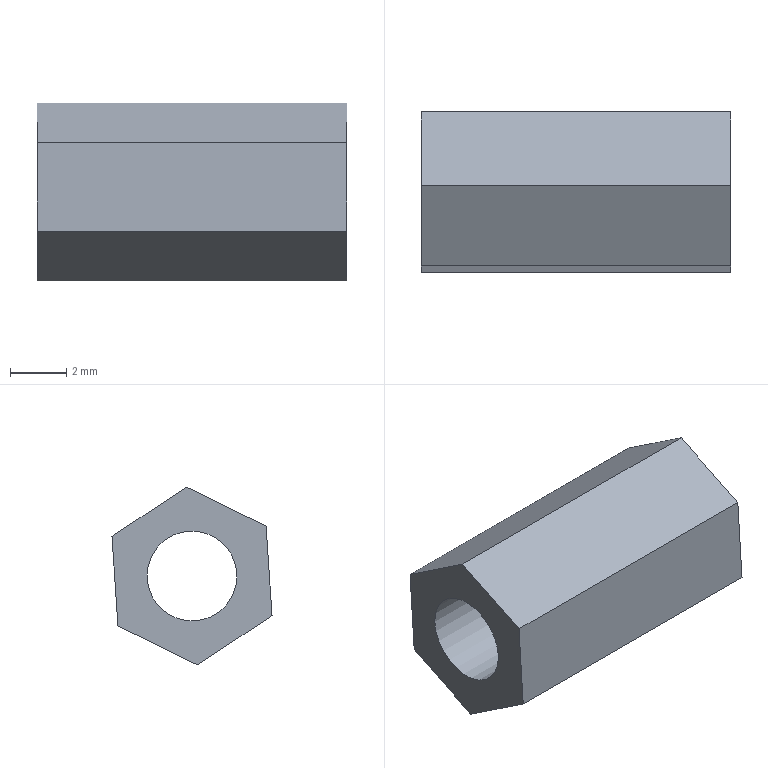Part | STEP file | Dodanie-wyci_gni_cie1_8 | 1 solid | 9 faces | box 11 x 5.689 x 6.325 mm | volume 198.638 mm3 | plane 8 | cylinder 1 | commonest cylinder face diameters 3.2 x1
STEP:
#1=CARTESIAN_POINT('',(0.,0.,0.));
#2=DIRECTION('',(0.,0.,1.));
#3=DIRECTION('',(1.,0.,0.));
#4=AXIS2_PLACEMENT_3D('',#1,#2,#3);
#5=CARTESIAN_POINT('',(142.868,119.819,-66.664));
#6=VERTEX_POINT('',#5);
#7=CARTESIAN_POINT('',(142.868,118.383,-67.37));
#8=DIRECTION('',(1.,0.,0.));
#9=DIRECTION('',(0.,0.8975,0.441));
#10=AXIS2_PLACEMENT_3D('',#7,#8,#9);
#11=CIRCLE('',#10,1.6);
#12=CARTESIAN_POINT('',(142.868,118.383,-67.37));
#13=DIRECTION('',(1.,0.,0.));
#14=DIRECTION('',(0.,0.8975,0.441));
#15=AXIS2_PLACEMENT_3D('',#12,#13,#14);
#16=CYLINDRICAL_SURFACE('',#15,1.6);
#17=CARTESIAN_POINT('',(0.,0.));
#18=DIRECTION('',(1.,0.));
#19=VECTOR('',#18,1.);
#20=LINE('',#17,#19);
#21=(GEOMETRIC_REPRESENTATION_CONTEXT(2)PARAMETRIC_REPRESENTATION_CONTEXT()REPRESENTATION_CONTEXT('',''));
#22=DEFINITIONAL_REPRESENTATION('',(#20),#21);
#23=PCURVE('',#16,#22);
#24=CARTESIAN_POINT('',(142.868,118.383,-67.37));
#25=DIRECTION('',(-1.,0.,0.));
#26=DIRECTION('',(0.,-0.8975,-0.441));
#27=AXIS2_PLACEMENT_3D('',#24,#25,#26);
#28=PLANE('',#27);
#29=CARTESIAN_POINT('',(-1.6,0.));
#30=CARTESIAN_POINT('',(-1.6,2.771));
#31=CARTESIAN_POINT('',(0.8,1.386));
#32=CARTESIAN_POINT('',(3.2,0.));
#33=CARTESIAN_POINT('',(0.8,-1.386));
#34=CARTESIAN_POINT('',(-1.6,-2.771));
#35=CARTESIAN_POINT('',(-1.6,0.));
#36=(BOUNDED_CURVE()B_SPLINE_CURVE(2,(#29,#30,#31,#32,#33,#34,#35),.UNSPECIFIED.,.T.,.F.)B_SPLINE_CURVE_WITH_KNOTS((1,2,2,2,2,1),(-2.094,0.,2.094,4.189,6.283,8.378),.UNSPECIFIED.)CURVE()GEOMETRIC_REPRESENTATION_ITEM()RATIONAL_B_SPLINE_CURVE((1.,0.5,1.,0.5,1.,0.5,1.))REPRESENTATION_ITEM(''));
#37=(GEOMETRIC_REPRESENTATION_CONTEXT(2)PARAMETRIC_REPRESENTATION_CONTEXT()REPRESENTATION_CONTEXT('',''));
#38=DEFINITIONAL_REPRESENTATION('',(#36),#37);
#39=PCURVE('',#28,#38);
#40=SURFACE_CURVE('',#11,(#23,#39),.PCURVE_S1.);
#41=EDGE_CURVE('',#6,#6,#40,.T.);
#42=ORIENTED_EDGE('',*,*,#41,.T.);
#43=CARTESIAN_POINT('',(153.868,119.819,-66.664));
#44=VERTEX_POINT('',#43);
#45=CARTESIAN_POINT('',(153.868,119.819,-66.664));
#46=DIRECTION('',(-1.,0.,0.));
#47=VECTOR('',#46,1.);
#48=LINE('',#45,#47);
#49=CARTESIAN_POINT('',(6.283,11.));
#50=DIRECTION('',(0.,-1.));
#51=VECTOR('',#50,1.);
#52=LINE('',#49,#51);
#53=(GEOMETRIC_REPRESENTATION_CONTEXT(2)PARAMETRIC_REPRESENTATION_CONTEXT()REPRESENTATION_CONTEXT('',''));
#54=DEFINITIONAL_REPRESENTATION('',(#52),#53);
#55=PCURVE('',#16,#54);
#56=CARTESIAN_POINT('',(0.,11.));
#57=DIRECTION('',(0.,-1.));
#58=VECTOR('',#57,1.);
#59=LINE('',#56,#58);
#60=(GEOMETRIC_REPRESENTATION_CONTEXT(2)PARAMETRIC_REPRESENTATION_CONTEXT()REPRESENTATION_CONTEXT('',''));
#61=DEFINITIONAL_REPRESENTATION('',(#59),#60);
#62=PCURVE('',#16,#61);
#63=SEAM_CURVE('',#48,(#55,#62),.PCURVE_S1.);
#64=EDGE_CURVE('',#44,#6,#63,.T.);
#65=ORIENTED_EDGE('',*,*,#64,.F.);
#66=CARTESIAN_POINT('',(153.868,118.383,-67.37));
#67=DIRECTION('',(-1.,0.,0.));
#68=DIRECTION('',(0.,0.8975,0.441));
#69=AXIS2_PLACEMENT_3D('',#66,#67,#68);
#70=CIRCLE('',#69,1.6);
#71=CARTESIAN_POINT('',(6.283,11.));
#72=DIRECTION('',(-1.,0.));
#73=VECTOR('',#72,1.);
#74=LINE('',#71,#73);
#75=(GEOMETRIC_REPRESENTATION_CONTEXT(2)PARAMETRIC_REPRESENTATION_CONTEXT()REPRESENTATION_CONTEXT('',''));
#76=DEFINITIONAL_REPRESENTATION('',(#74),#75);
#77=PCURVE('',#16,#76);
#78=CARTESIAN_POINT('',(153.868,118.383,-67.37));
#79=DIRECTION('',(-1.,0.,0.));
#80=DIRECTION('',(0.,-0.8975,-0.441));
#81=AXIS2_PLACEMENT_3D('',#78,#79,#80);
#82=PLANE('',#81);
#83=CARTESIAN_POINT('',(0.,0.));
#84=DIRECTION('',(-1.,0.));
#85=AXIS2_PLACEMENT_2D('',#83,#84);
#86=CIRCLE('',#85,1.6);
#87=(GEOMETRIC_REPRESENTATION_CONTEXT(2)PARAMETRIC_REPRESENTATION_CONTEXT()REPRESENTATION_CONTEXT('',''));
#88=DEFINITIONAL_REPRESENTATION('',(#86),#87);
#89=PCURVE('',#82,#88);
#90=SURFACE_CURVE('',#70,(#77,#89),.PCURVE_S1.);
#91=EDGE_CURVE('',#44,#44,#90,.T.);
#92=ORIENTED_EDGE('',*,*,#91,.T.);
#93=ORIENTED_EDGE('',*,*,#64,.T.);
#94=EDGE_LOOP('',(#42,#65,#92,#93));
#95=FACE_BOUND('',#94,.F.);
#96=ADVANCED_FACE('',(#95),#16,.F.);
#97=ORIENTED_EDGE('',*,*,#91,.T.);
#98=EDGE_LOOP('',(#97));
#99=FACE_BOUND('',#98,.T.);
#100=CARTESIAN_POINT('',(153.868,115.75,-65.605));
#101=VERTEX_POINT('',#100);
#102=CARTESIAN_POINT('',(153.868,118.595,-64.207));
#103=VERTEX_POINT('',#102);
#104=CARTESIAN_POINT('',(153.868,115.75,-65.605));
#105=DIRECTION('',(0.,0.8975,0.441));
#106=VECTOR('',#105,1.);
#107=LINE('',#104,#106);
#108=CARTESIAN_POINT('',(1.585,2.745));
#109=DIRECTION('',(-1.,0.));
#110=VECTOR('',#109,1.);
#111=LINE('',#108,#110);
#112=(GEOMETRIC_REPRESENTATION_CONTEXT(2)PARAMETRIC_REPRESENTATION_CONTEXT()REPRESENTATION_CONTEXT('',''));
#113=DEFINITIONAL_REPRESENTATION('',(#111),#112);
#114=PCURVE('',#82,#113);
#115=CARTESIAN_POINT('',(148.368,117.172,-64.906));
#116=DIRECTION('',(0.,0.441,-0.8975));
#117=DIRECTION('',(0.,-0.8975,-0.441));
#118=AXIS2_PLACEMENT_3D('',#115,#116,#117);
#119=PLANE('',#118);
#120=CARTESIAN_POINT('',(1.585,-5.5));
#121=DIRECTION('',(-1.,0.));
#122=VECTOR('',#121,1.);
#123=LINE('',#120,#122);
#124=(GEOMETRIC_REPRESENTATION_CONTEXT(2)PARAMETRIC_REPRESENTATION_CONTEXT()REPRESENTATION_CONTEXT('',''));
#125=DEFINITIONAL_REPRESENTATION('',(#123),#124);
#126=PCURVE('',#119,#125);
#127=SURFACE_CURVE('',#107,(#114,#126),.PCURVE_S1.);
#128=EDGE_CURVE('',#101,#103,#127,.T.);
#129=ORIENTED_EDGE('',*,*,#128,.F.);
#130=CARTESIAN_POINT('',(153.868,115.538,-68.768));
#131=VERTEX_POINT('',#130);
#132=CARTESIAN_POINT('',(153.868,115.538,-68.768));
#133=DIRECTION('',(0.,0.0668,0.9978));
#134=VECTOR('',#133,1.);
#135=LINE('',#132,#134);
#136=CARTESIAN_POINT('',(3.17,-0.000000001));
#137=DIRECTION('',(-0.5,0.866));
#138=VECTOR('',#137,1.);
#139=LINE('',#136,#138);
#140=(GEOMETRIC_REPRESENTATION_CONTEXT(2)PARAMETRIC_REPRESENTATION_CONTEXT()REPRESENTATION_CONTEXT('',''));
#141=DEFINITIONAL_REPRESENTATION('',(#139),#140);
#142=PCURVE('',#82,#141);
#143=CARTESIAN_POINT('',(148.368,115.644,-67.187));
#144=DIRECTION('',(0.,0.9978,-0.0668));
#145=DIRECTION('',(0.,-0.0668,-0.9978));
#146=AXIS2_PLACEMENT_3D('',#143,#144,#145);
#147=PLANE('',#146);
#148=CARTESIAN_POINT('',(1.585,-5.5));
#149=DIRECTION('',(-1.,0.));
#150=VECTOR('',#149,1.);
#151=LINE('',#148,#150);
#152=(GEOMETRIC_REPRESENTATION_CONTEXT(2)PARAMETRIC_REPRESENTATION_CONTEXT()REPRESENTATION_CONTEXT('',''));
#153=DEFINITIONAL_REPRESENTATION('',(#151),#152);
#154=PCURVE('',#147,#153);
#155=SURFACE_CURVE('',#135,(#142,#154),.PCURVE_S1.);
#156=EDGE_CURVE('',#131,#101,#155,.T.);
#157=ORIENTED_EDGE('',*,*,#156,.F.);
#158=CARTESIAN_POINT('',(153.868,118.171,-70.532));
#159=VERTEX_POINT('',#158);
#160=CARTESIAN_POINT('',(153.868,118.171,-70.532));
#161=DIRECTION('',(0.,-0.8307,0.5567));
#162=VECTOR('',#161,1.);
#163=LINE('',#160,#162);
#164=CARTESIAN_POINT('',(1.585,-2.745));
#165=DIRECTION('',(0.5,0.866));
#166=VECTOR('',#165,1.);
#167=LINE('',#164,#166);
#168=(GEOMETRIC_REPRESENTATION_CONTEXT(2)PARAMETRIC_REPRESENTATION_CONTEXT()REPRESENTATION_CONTEXT('',''));
#169=DEFINITIONAL_REPRESENTATION('',(#167),#168);
#170=PCURVE('',#82,#169);
#171=CARTESIAN_POINT('',(148.368,116.855,-69.65));
#172=DIRECTION('',(0.,0.5567,0.8307));
#173=DIRECTION('',(0.,0.8307,-0.5567));
#174=AXIS2_PLACEMENT_3D('',#171,#172,#173);
#175=PLANE('',#174);
#176=CARTESIAN_POINT('',(1.585,-5.5));
#177=DIRECTION('',(-1.,0.));
#178=VECTOR('',#177,1.);
#179=LINE('',#176,#178);
#180=(GEOMETRIC_REPRESENTATION_CONTEXT(2)PARAMETRIC_REPRESENTATION_CONTEXT()REPRESENTATION_CONTEXT('',''));
#181=DEFINITIONAL_REPRESENTATION('',(#179),#180);
#182=PCURVE('',#175,#181);
#183=SURFACE_CURVE('',#163,(#170,#182),.PCURVE_S1.);
#184=EDGE_CURVE('',#159,#131,#183,.T.);
#185=ORIENTED_EDGE('',*,*,#184,.F.);
#186=CARTESIAN_POINT('',(153.868,121.016,-69.134));
#187=VERTEX_POINT('',#186);
#188=CARTESIAN_POINT('',(153.868,121.016,-69.134));
#189=DIRECTION('',(0.,-0.8975,-0.441));
#190=VECTOR('',#189,1.);
#191=LINE('',#188,#190);
#192=CARTESIAN_POINT('',(-1.585,-2.745));
#193=DIRECTION('',(1.,0.));
#194=VECTOR('',#193,1.);
#195=LINE('',#192,#194);
#196=(GEOMETRIC_REPRESENTATION_CONTEXT(2)PARAMETRIC_REPRESENTATION_CONTEXT()REPRESENTATION_CONTEXT('',''));
#197=DEFINITIONAL_REPRESENTATION('',(#195),#196);
#198=PCURVE('',#82,#197);
#199=CARTESIAN_POINT('',(148.368,119.594,-69.833));
#200=DIRECTION('',(0.,-0.441,0.8975));
#201=DIRECTION('',(0.,0.8975,0.441));
#202=AXIS2_PLACEMENT_3D('',#199,#200,#201);
#203=PLANE('',#202);
#204=CARTESIAN_POINT('',(1.585,-5.5));
#205=DIRECTION('',(-1.,0.));
#206=VECTOR('',#205,1.);
#207=LINE('',#204,#206);
#208=(GEOMETRIC_REPRESENTATION_CONTEXT(2)PARAMETRIC_REPRESENTATION_CONTEXT()REPRESENTATION_CONTEXT('',''));
#209=DEFINITIONAL_REPRESENTATION('',(#207),#208);
#210=PCURVE('',#203,#209);
#211=SURFACE_CURVE('',#191,(#198,#210),.PCURVE_S1.);
#212=EDGE_CURVE('',#187,#159,#211,.T.);
#213=ORIENTED_EDGE('',*,*,#212,.F.);
#214=CARTESIAN_POINT('',(153.868,121.228,-65.972));
#215=VERTEX_POINT('',#214);
#216=CARTESIAN_POINT('',(153.868,121.228,-65.972));
#217=DIRECTION('',(0.,-0.0668,-0.9978));
#218=VECTOR('',#217,1.);
#219=LINE('',#216,#218);
#220=CARTESIAN_POINT('',(-3.17,0.000000001));
#221=DIRECTION('',(0.5,-0.866));
#222=VECTOR('',#221,1.);
#223=LINE('',#220,#222);
#224=(GEOMETRIC_REPRESENTATION_CONTEXT(2)PARAMETRIC_REPRESENTATION_CONTEXT()REPRESENTATION_CONTEXT('',''));
#225=DEFINITIONAL_REPRESENTATION('',(#223),#224);
#226=PCURVE('',#82,#225);
#227=CARTESIAN_POINT('',(148.368,121.122,-67.553));
#228=DIRECTION('',(0.,-0.9978,0.0668));
#229=DIRECTION('',(0.,0.0668,0.9978));
#230=AXIS2_PLACEMENT_3D('',#227,#228,#229);
#231=PLANE('',#230);
#232=CARTESIAN_POINT('',(1.585,-5.5));
#233=DIRECTION('',(-1.,0.));
#234=VECTOR('',#233,1.);
#235=LINE('',#232,#234);
#236=(GEOMETRIC_REPRESENTATION_CONTEXT(2)PARAMETRIC_REPRESENTATION_CONTEXT()REPRESENTATION_CONTEXT('',''));
#237=DEFINITIONAL_REPRESENTATION('',(#235),#236);
#238=PCURVE('',#231,#237);
#239=SURFACE_CURVE('',#219,(#226,#238),.PCURVE_S1.);
#240=EDGE_CURVE('',#215,#187,#239,.T.);
#241=ORIENTED_EDGE('',*,*,#240,.F.);
#242=CARTESIAN_POINT('',(153.868,118.595,-64.207));
#243=DIRECTION('',(0.,0.8307,-0.5567));
#244=VECTOR('',#243,1.);
#245=LINE('',#242,#244);
#246=CARTESIAN_POINT('',(-1.585,2.745));
#247=DIRECTION('',(-0.5,-0.866));
#248=VECTOR('',#247,1.);
#249=LINE('',#246,#248);
#250=(GEOMETRIC_REPRESENTATION_CONTEXT(2)PARAMETRIC_REPRESENTATION_CONTEXT()REPRESENTATION_CONTEXT('',''));
#251=DEFINITIONAL_REPRESENTATION('',(#249),#250);
#252=PCURVE('',#82,#251);
#253=CARTESIAN_POINT('',(148.368,119.911,-65.09));
#254=DIRECTION('',(0.,-0.5567,-0.8307));
#255=DIRECTION('',(0.,-0.8307,0.5567));
#256=AXIS2_PLACEMENT_3D('',#253,#254,#255);
#257=PLANE('',#256);
#258=CARTESIAN_POINT('',(1.585,-5.5));
#259=DIRECTION('',(-1.,0.));
#260=VECTOR('',#259,1.);
#261=LINE('',#258,#260);
#262=(GEOMETRIC_REPRESENTATION_CONTEXT(2)PARAMETRIC_REPRESENTATION_CONTEXT()REPRESENTATION_CONTEXT('',''));
#263=DEFINITIONAL_REPRESENTATION('',(#261),#262);
#264=PCURVE('',#257,#263);
#265=SURFACE_CURVE('',#245,(#252,#264),.PCURVE_S1.);
#266=EDGE_CURVE('',#103,#215,#265,.T.);
#267=ORIENTED_EDGE('',*,*,#266,.F.);
#268=EDGE_LOOP('',(#129,#157,#185,#213,#241,#267));
#269=FACE_BOUND('',#268,.T.);
#270=ADVANCED_FACE('',(#99,#269),#82,.F.);
#271=ORIENTED_EDGE('',*,*,#41,.T.);
#272=EDGE_LOOP('',(#271));
#273=FACE_BOUND('',#272,.T.);
#274=CARTESIAN_POINT('',(142.868,115.538,-68.768));
#275=VERTEX_POINT('',#274);
#276=CARTESIAN_POINT('',(142.868,115.75,-65.605));
#277=VERTEX_POINT('',#276);
#278=CARTESIAN_POINT('',(142.868,115.538,-68.768));
#279=DIRECTION('',(0.,0.0668,0.9978));
#280=VECTOR('',#279,1.);
#281=LINE('',#278,#280);
#282=CARTESIAN_POINT('',(3.17,-0.000000001));
#283=DIRECTION('',(-0.5,0.866));
#284=VECTOR('',#283,1.);
#285=LINE('',#282,#284);
#286=(GEOMETRIC_REPRESENTATION_CONTEXT(2)PARAMETRIC_REPRESENTATION_CONTEXT()REPRESENTATION_CONTEXT('',''));
#287=DEFINITIONAL_REPRESENTATION('',(#285),#286);
#288=PCURVE('',#28,#287);
#289=CARTESIAN_POINT('',(1.585,5.5));
#290=DIRECTION('',(-1.,0.));
#291=VECTOR('',#290,1.);
#292=LINE('',#289,#291);
#293=(GEOMETRIC_REPRESENTATION_CONTEXT(2)PARAMETRIC_REPRESENTATION_CONTEXT()REPRESENTATION_CONTEXT('',''));
#294=DEFINITIONAL_REPRESENTATION('',(#292),#293);
#295=PCURVE('',#147,#294);
#296=SURFACE_CURVE('',#281,(#288,#295),.PCURVE_S1.);
#297=EDGE_CURVE('',#275,#277,#296,.T.);
#298=ORIENTED_EDGE('',*,*,#297,.T.);
#299=CARTESIAN_POINT('',(142.868,118.595,-64.207));
#300=VERTEX_POINT('',#299);
#301=CARTESIAN_POINT('',(142.868,115.75,-65.605));
#302=DIRECTION('',(0.,0.8975,0.441));
#303=VECTOR('',#302,1.);
#304=LINE('',#301,#303);
#305=CARTESIAN_POINT('',(1.585,2.745));
#306=DIRECTION('',(-1.,0.));
#307=VECTOR('',#306,1.);
#308=LINE('',#305,#307);
#309=(GEOMETRIC_REPRESENTATION_CONTEXT(2)PARAMETRIC_REPRESENTATION_CONTEXT()REPRESENTATION_CONTEXT('',''));
#310=DEFINITIONAL_REPRESENTATION('',(#308),#309);
#311=PCURVE('',#28,#310);
#312=CARTESIAN_POINT('',(1.585,5.5));
#313=DIRECTION('',(-1.,0.));
#314=VECTOR('',#313,1.);
#315=LINE('',#312,#314);
#316=(GEOMETRIC_REPRESENTATION_CONTEXT(2)PARAMETRIC_REPRESENTATION_CONTEXT()REPRESENTATION_CONTEXT('',''));
#317=DEFINITIONAL_REPRESENTATION('',(#315),#316);
#318=PCURVE('',#119,#317);
#319=SURFACE_CURVE('',#304,(#311,#318),.PCURVE_S1.);
#320=EDGE_CURVE('',#277,#300,#319,.T.);
#321=ORIENTED_EDGE('',*,*,#320,.T.);
#322=CARTESIAN_POINT('',(142.868,121.228,-65.972));
#323=VERTEX_POINT('',#322);
#324=CARTESIAN_POINT('',(142.868,118.595,-64.207));
#325=DIRECTION('',(0.,0.8307,-0.5567));
#326=VECTOR('',#325,1.);
#327=LINE('',#324,#326);
#328=CARTESIAN_POINT('',(-1.585,2.745));
#329=DIRECTION('',(-0.5,-0.866));
#330=VECTOR('',#329,1.);
#331=LINE('',#328,#330);
#332=(GEOMETRIC_REPRESENTATION_CONTEXT(2)PARAMETRIC_REPRESENTATION_CONTEXT()REPRESENTATION_CONTEXT('',''));
#333=DEFINITIONAL_REPRESENTATION('',(#331),#332);
#334=PCURVE('',#28,#333);
#335=CARTESIAN_POINT('',(1.585,5.5));
#336=DIRECTION('',(-1.,0.));
#337=VECTOR('',#336,1.);
#338=LINE('',#335,#337);
#339=(GEOMETRIC_REPRESENTATION_CONTEXT(2)PARAMETRIC_REPRESENTATION_CONTEXT()REPRESENTATION_CONTEXT('',''));
#340=DEFINITIONAL_REPRESENTATION('',(#338),#339);
#341=PCURVE('',#257,#340);
#342=SURFACE_CURVE('',#327,(#334,#341),.PCURVE_S1.);
#343=EDGE_CURVE('',#300,#323,#342,.T.);
#344=ORIENTED_EDGE('',*,*,#343,.T.);
#345=CARTESIAN_POINT('',(142.868,121.016,-69.134));
#346=VERTEX_POINT('',#345);
#347=CARTESIAN_POINT('',(142.868,121.228,-65.972));
#348=DIRECTION('',(0.,-0.0668,-0.9978));
#349=VECTOR('',#348,1.);
#350=LINE('',#347,#349);
#351=CARTESIAN_POINT('',(-3.17,0.000000001));
#352=DIRECTION('',(0.5,-0.866));
#353=VECTOR('',#352,1.);
#354=LINE('',#351,#353);
#355=(GEOMETRIC_REPRESENTATION_CONTEXT(2)PARAMETRIC_REPRESENTATION_CONTEXT()REPRESENTATION_CONTEXT('',''));
#356=DEFINITIONAL_REPRESENTATION('',(#354),#355);
#357=PCURVE('',#28,#356);
#358=CARTESIAN_POINT('',(1.585,5.5));
#359=DIRECTION('',(-1.,0.));
#360=VECTOR('',#359,1.);
#361=LINE('',#358,#360);
#362=(GEOMETRIC_REPRESENTATION_CONTEXT(2)PARAMETRIC_REPRESENTATION_CONTEXT()REPRESENTATION_CONTEXT('',''));
#363=DEFINITIONAL_REPRESENTATION('',(#361),#362);
#364=PCURVE('',#231,#363);
#365=SURFACE_CURVE('',#350,(#357,#364),.PCURVE_S1.);
#366=EDGE_CURVE('',#323,#346,#365,.T.);
#367=ORIENTED_EDGE('',*,*,#366,.T.);
#368=CARTESIAN_POINT('',(142.868,118.171,-70.532));
#369=VERTEX_POINT('',#368);
#370=CARTESIAN_POINT('',(142.868,121.016,-69.134));
#371=DIRECTION('',(0.,-0.8975,-0.441));
#372=VECTOR('',#371,1.);
#373=LINE('',#370,#372);
#374=CARTESIAN_POINT('',(-1.585,-2.745));
#375=DIRECTION('',(1.,0.));
#376=VECTOR('',#375,1.);
#377=LINE('',#374,#376);
#378=(GEOMETRIC_REPRESENTATION_CONTEXT(2)PARAMETRIC_REPRESENTATION_CONTEXT()REPRESENTATION_CONTEXT('',''));
#379=DEFINITIONAL_REPRESENTATION('',(#377),#378);
#380=PCURVE('',#28,#379);
#381=CARTESIAN_POINT('',(1.585,5.5));
#382=DIRECTION('',(-1.,0.));
#383=VECTOR('',#382,1.);
#384=LINE('',#381,#383);
#385=(GEOMETRIC_REPRESENTATION_CONTEXT(2)PARAMETRIC_REPRESENTATION_CONTEXT()REPRESENTATION_CONTEXT('',''));
#386=DEFINITIONAL_REPRESENTATION('',(#384),#385);
#387=PCURVE('',#203,#386);
#388=SURFACE_CURVE('',#373,(#380,#387),.PCURVE_S1.);
#389=EDGE_CURVE('',#346,#369,#388,.T.);
#390=ORIENTED_EDGE('',*,*,#389,.T.);
#391=CARTESIAN_POINT('',(142.868,118.171,-70.532));
#392=DIRECTION('',(0.,-0.8307,0.5567));
#393=VECTOR('',#392,1.);
#394=LINE('',#391,#393);
#395=CARTESIAN_POINT('',(1.585,-2.745));
#396=DIRECTION('',(0.5,0.866));
#397=VECTOR('',#396,1.);
#398=LINE('',#395,#397);
#399=(GEOMETRIC_REPRESENTATION_CONTEXT(2)PARAMETRIC_REPRESENTATION_CONTEXT()REPRESENTATION_CONTEXT('',''));
#400=DEFINITIONAL_REPRESENTATION('',(#398),#399);
#401=PCURVE('',#28,#400);
#402=CARTESIAN_POINT('',(1.585,5.5));
#403=DIRECTION('',(-1.,0.));
#404=VECTOR('',#403,1.);
#405=LINE('',#402,#404);
#406=(GEOMETRIC_REPRESENTATION_CONTEXT(2)PARAMETRIC_REPRESENTATION_CONTEXT()REPRESENTATION_CONTEXT('',''));
#407=DEFINITIONAL_REPRESENTATION('',(#405),#406);
#408=PCURVE('',#175,#407);
#409=SURFACE_CURVE('',#394,(#401,#408),.PCURVE_S1.);
#410=EDGE_CURVE('',#369,#275,#409,.T.);
#411=ORIENTED_EDGE('',*,*,#410,.T.);
#412=EDGE_LOOP('',(#298,#321,#344,#367,#390,#411));
#413=FACE_BOUND('',#412,.T.);
#414=ADVANCED_FACE('',(#273,#413),#28,.T.);
#415=CARTESIAN_POINT('',(142.868,121.228,-65.972));
#416=DIRECTION('',(1.,0.,0.));
#417=VECTOR('',#416,1.);
#418=LINE('',#415,#417);
#419=CARTESIAN_POINT('',(-1.585,5.5));
#420=DIRECTION('',(0.,-1.));
#421=VECTOR('',#420,1.);
#422=LINE('',#419,#421);
#423=(GEOMETRIC_REPRESENTATION_CONTEXT(2)PARAMETRIC_REPRESENTATION_CONTEXT()REPRESENTATION_CONTEXT('',''));
#424=DEFINITIONAL_REPRESENTATION('',(#422),#423);
#425=PCURVE('',#257,#424);
#426=CARTESIAN_POINT('',(1.585,5.5));
#427=DIRECTION('',(0.,-1.));
#428=VECTOR('',#427,1.);
#429=LINE('',#426,#428);
#430=(GEOMETRIC_REPRESENTATION_CONTEXT(2)PARAMETRIC_REPRESENTATION_CONTEXT()REPRESENTATION_CONTEXT('',''));
#431=DEFINITIONAL_REPRESENTATION('',(#429),#430);
#432=PCURVE('',#231,#431);
#433=SURFACE_CURVE('',#418,(#425,#432),.PCURVE_S1.);
#434=EDGE_CURVE('',#323,#215,#433,.T.);
#435=ORIENTED_EDGE('',*,*,#434,.F.);
#436=ORIENTED_EDGE('',*,*,#343,.F.);
#437=CARTESIAN_POINT('',(153.868,118.595,-64.207));
#438=DIRECTION('',(-1.,0.,0.));
#439=VECTOR('',#438,1.);
#440=LINE('',#437,#439);
#441=CARTESIAN_POINT('',(1.585,-5.5));
#442=DIRECTION('',(0.,1.));
#443=VECTOR('',#442,1.);
#444=LINE('',#441,#443);
#445=(GEOMETRIC_REPRESENTATION_CONTEXT(2)PARAMETRIC_REPRESENTATION_CONTEXT()REPRESENTATION_CONTEXT('',''));
#446=DEFINITIONAL_REPRESENTATION('',(#444),#445);
#447=PCURVE('',#257,#446);
#448=CARTESIAN_POINT('',(-1.585,-5.5));
#449=DIRECTION('',(0.,1.));
#450=VECTOR('',#449,1.);
#451=LINE('',#448,#450);
#452=(GEOMETRIC_REPRESENTATION_CONTEXT(2)PARAMETRIC_REPRESENTATION_CONTEXT()REPRESENTATION_CONTEXT('',''));
#453=DEFINITIONAL_REPRESENTATION('',(#451),#452);
#454=PCURVE('',#119,#453);
#455=SURFACE_CURVE('',#440,(#447,#454),.PCURVE_S1.);
#456=EDGE_CURVE('',#103,#300,#455,.T.);
#457=ORIENTED_EDGE('',*,*,#456,.F.);
#458=ORIENTED_EDGE('',*,*,#266,.T.);
#459=EDGE_LOOP('',(#435,#436,#457,#458));
#460=FACE_BOUND('',#459,.T.);
#461=ADVANCED_FACE('',(#460),#257,.F.);
#462=ORIENTED_EDGE('',*,*,#456,.T.);
#463=ORIENTED_EDGE('',*,*,#320,.F.);
#464=CARTESIAN_POINT('',(153.868,115.75,-65.605));
#465=DIRECTION('',(-1.,0.,0.));
#466=VECTOR('',#465,1.);
#467=LINE('',#464,#466);
#468=CARTESIAN_POINT('',(1.585,-5.5));
#469=DIRECTION('',(0.,1.));
#470=VECTOR('',#469,1.);
#471=LINE('',#468,#470);
#472=(GEOMETRIC_REPRESENTATION_CONTEXT(2)PARAMETRIC_REPRESENTATION_CONTEXT()REPRESENTATION_CONTEXT('',''));
#473=DEFINITIONAL_REPRESENTATION('',(#471),#472);
#474=PCURVE('',#119,#473);
#475=CARTESIAN_POINT('',(-1.585,-5.5));
#476=DIRECTION('',(0.,1.));
#477=VECTOR('',#476,1.);
#478=LINE('',#475,#477);
#479=(GEOMETRIC_REPRESENTATION_CONTEXT(2)PARAMETRIC_REPRESENTATION_CONTEXT()REPRESENTATION_CONTEXT('',''));
#480=DEFINITIONAL_REPRESENTATION('',(#478),#479);
#481=PCURVE('',#147,#480);
#482=SURFACE_CURVE('',#467,(#474,#481),.PCURVE_S1.);
#483=EDGE_CURVE('',#101,#277,#482,.T.);
#484=ORIENTED_EDGE('',*,*,#483,.F.);
#485=ORIENTED_EDGE('',*,*,#128,.T.);
#486=EDGE_LOOP('',(#462,#463,#484,#485));
#487=FACE_BOUND('',#486,.T.);
#488=ADVANCED_FACE('',(#487),#119,.F.);
#489=ORIENTED_EDGE('',*,*,#483,.T.);
#490=ORIENTED_EDGE('',*,*,#297,.F.);
#491=CARTESIAN_POINT('',(153.868,115.538,-68.768));
#492=DIRECTION('',(-1.,0.,0.));
#493=VECTOR('',#492,1.);
#494=LINE('',#491,#493);
#495=CARTESIAN_POINT('',(1.585,-5.5));
#496=DIRECTION('',(0.,1.));
#497=VECTOR('',#496,1.);
#498=LINE('',#495,#497);
#499=(GEOMETRIC_REPRESENTATION_CONTEXT(2)PARAMETRIC_REPRESENTATION_CONTEXT()REPRESENTATION_CONTEXT('',''));
#500=DEFINITIONAL_REPRESENTATION('',(#498),#499);
#501=PCURVE('',#147,#500);
#502=CARTESIAN_POINT('',(-1.585,-5.5));
#503=DIRECTION('',(0.,1.));
#504=VECTOR('',#503,1.);
#505=LINE('',#502,#504);
#506=(GEOMETRIC_REPRESENTATION_CONTEXT(2)PARAMETRIC_REPRESENTATION_CONTEXT()REPRESENTATION_CONTEXT('',''));
#507=DEFINITIONAL_REPRESENTATION('',(#505),#506);
#508=PCURVE('',#175,#507);
#509=SURFACE_CURVE('',#494,(#501,#508),.PCURVE_S1.);
#510=EDGE_CURVE('',#131,#275,#509,.T.);
#511=ORIENTED_EDGE('',*,*,#510,.F.);
#512=ORIENTED_EDGE('',*,*,#156,.T.);
#513=EDGE_LOOP('',(#489,#490,#511,#512));
#514=FACE_BOUND('',#513,.T.);
#515=ADVANCED_FACE('',(#514),#147,.F.);
#516=ORIENTED_EDGE('',*,*,#510,.T.);
#517=ORIENTED_EDGE('',*,*,#410,.F.);
#518=CARTESIAN_POINT('',(153.868,118.171,-70.532));
#519=DIRECTION('',(-1.,0.,0.));
#520=VECTOR('',#519,1.);
#521=LINE('',#518,#520);
#522=CARTESIAN_POINT('',(1.585,-5.5));
#523=DIRECTION('',(0.,1.));
#524=VECTOR('',#523,1.);
#525=LINE('',#522,#524);
#526=(GEOMETRIC_REPRESENTATION_CONTEXT(2)PARAMETRIC_REPRESENTATION_CONTEXT()REPRESENTATION_CONTEXT('',''));
#527=DEFINITIONAL_REPRESENTATION('',(#525),#526);
#528=PCURVE('',#175,#527);
#529=CARTESIAN_POINT('',(-1.585,-5.5));
#530=DIRECTION('',(0.,1.));
#531=VECTOR('',#530,1.);
#532=LINE('',#529,#531);
#533=(GEOMETRIC_REPRESENTATION_CONTEXT(2)PARAMETRIC_REPRESENTATION_CONTEXT()REPRESENTATION_CONTEXT('',''));
#534=DEFINITIONAL_REPRESENTATION('',(#532),#533);
#535=PCURVE('',#203,#534);
#536=SURFACE_CURVE('',#521,(#528,#535),.PCURVE_S1.);
#537=EDGE_CURVE('',#159,#369,#536,.T.);
#538=ORIENTED_EDGE('',*,*,#537,.F.);
#539=ORIENTED_EDGE('',*,*,#184,.T.);
#540=EDGE_LOOP('',(#516,#517,#538,#539));
#541=FACE_BOUND('',#540,.T.);
#542=ADVANCED_FACE('',(#541),#175,.F.);
#543=ORIENTED_EDGE('',*,*,#537,.T.);
#544=ORIENTED_EDGE('',*,*,#389,.F.);
#545=CARTESIAN_POINT('',(153.868,121.016,-69.134));
#546=DIRECTION('',(-1.,0.,0.));
#547=VECTOR('',#546,1.);
#548=LINE('',#545,#547);
#549=CARTESIAN_POINT('',(1.585,-5.5));
#550=DIRECTION('',(0.,1.));
#551=VECTOR('',#550,1.);
#552=LINE('',#549,#551);
#553=(GEOMETRIC_REPRESENTATION_CONTEXT(2)PARAMETRIC_REPRESENTATION_CONTEXT()REPRESENTATION_CONTEXT('',''));
#554=DEFINITIONAL_REPRESENTATION('',(#552),#553);
#555=PCURVE('',#203,#554);
#556=CARTESIAN_POINT('',(-1.585,-5.5));
#557=DIRECTION('',(0.,1.));
#558=VECTOR('',#557,1.);
#559=LINE('',#556,#558);
#560=(GEOMETRIC_REPRESENTATION_CONTEXT(2)PARAMETRIC_REPRESENTATION_CONTEXT()REPRESENTATION_CONTEXT('',''));
#561=DEFINITIONAL_REPRESENTATION('',(#559),#560);
#562=PCURVE('',#231,#561);
#563=SURFACE_CURVE('',#548,(#555,#562),.PCURVE_S1.);
#564=EDGE_CURVE('',#187,#346,#563,.T.);
#565=ORIENTED_EDGE('',*,*,#564,.F.);
#566=ORIENTED_EDGE('',*,*,#212,.T.);
#567=EDGE_LOOP('',(#543,#544,#565,#566));
#568=FACE_BOUND('',#567,.T.);
#569=ADVANCED_FACE('',(#568),#203,.F.);
#570=ORIENTED_EDGE('',*,*,#564,.T.);
#571=ORIENTED_EDGE('',*,*,#366,.F.);
#572=ORIENTED_EDGE('',*,*,#434,.T.);
#573=ORIENTED_EDGE('',*,*,#240,.T.);
#574=EDGE_LOOP('',(#570,#571,#572,#573));
#575=FACE_BOUND('',#574,.T.);
#576=ADVANCED_FACE('',(#575),#231,.F.);
#577=CLOSED_SHELL('',(#96,#270,#414,#461,#488,#515,#542,#569,#576));
#578=MANIFOLD_SOLID_BREP('',#577);
#579=(LENGTH_UNIT()NAMED_UNIT(*)SI_UNIT(.MILLI.,.METRE.));
#580=UNCERTAINTY_MEASURE_WITH_UNIT(LENGTH_MEASURE(0.0000001),#579,'','');
#581=(NAMED_UNIT(*)PLANE_ANGLE_UNIT()SI_UNIT($,.RADIAN.));
#582=(NAMED_UNIT(*)SI_UNIT($,.STERADIAN.)SOLID_ANGLE_UNIT());
#583=(GEOMETRIC_REPRESENTATION_CONTEXT(3)GLOBAL_UNCERTAINTY_ASSIGNED_CONTEXT((#580))GLOBAL_UNIT_ASSIGNED_CONTEXT((#579,#581,#582))REPRESENTATION_CONTEXT('',''));
#584=ADVANCED_BREP_SHAPE_REPRESENTATION('',(#4,#578),#583);